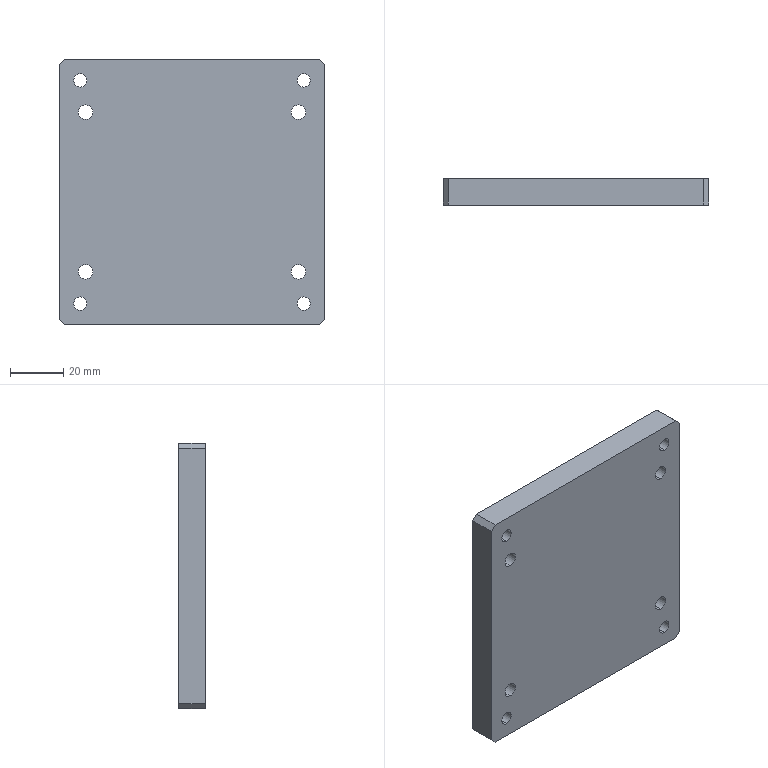Part | STEP file | PN_0037 vibratory adjusting plate B | 1 solid | 38 faces | box 100 x 10 x 100 mm | volume 97001 mm3 | cylinder 24 | plane 14 | commonest cylinder face diameters 5 x8 5.5 x8 10 x8